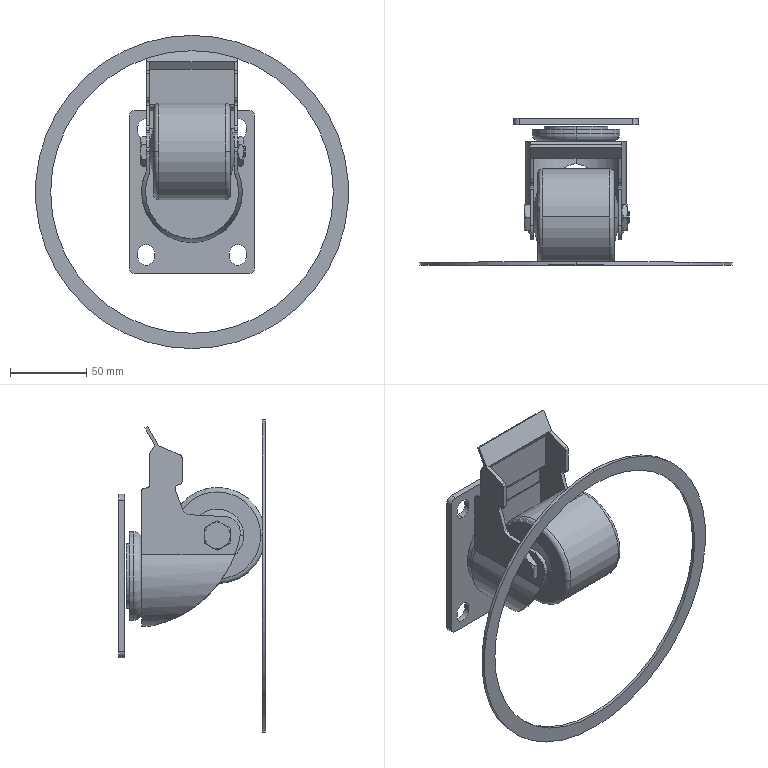Part | SolidWorks | features BaseBody 4, BossThin 1 | 5 solids | 157 faces | box 204.978 x 96 x 204.978 mm | volume 270055 mm3 | plane 70 | cylinder 54 | cone 27 | torus 6 | commonest cylinder face diameters 11 x12 4 x10 8 x6 10 x2 20 x2 25 x2